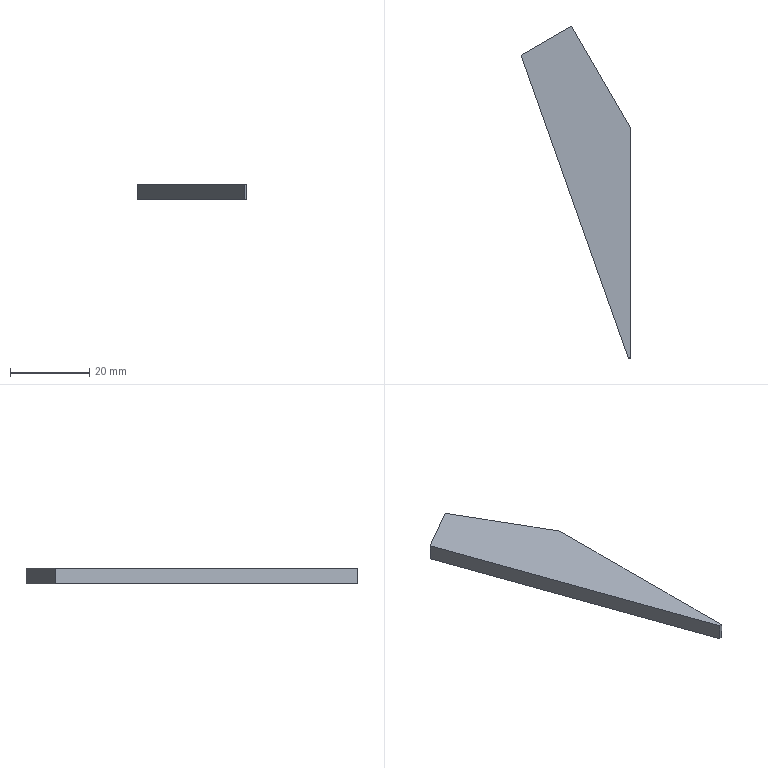Part | STEP file | Cable Chain Bracket-1 | 1 solid | 7 faces | box 27.758 x 83.881 x 4 mm | volume 4206 mm3 | plane 7
STEP:
#1=CARTESIAN_POINT('',(-31.538,-58.869,-4.));
#2=VERTEX_POINT('',#1);
#3=CARTESIAN_POINT('',(-32.245,-58.869,-4.));
#4=VERTEX_POINT('',#3);
#5=CARTESIAN_POINT('',(-32.245,-58.869,-4.));
#6=DIRECTION('',(-1.,0.,0.));
#7=VECTOR('',#6,1000.);
#8=LINE('',#5,#7);
#9=EDGE_CURVE('',#2,#4,#8,.T.);
#10=ORIENTED_EDGE('',*,*,#9,.T.);
#11=CARTESIAN_POINT('',(-59.295,17.646,-4.));
#12=VERTEX_POINT('',#11);
#13=CARTESIAN_POINT('',(-59.295,17.646,-4.));
#14=DIRECTION('',(0.3333,-0.9428,0.));
#15=VECTOR('',#14,1000.);
#16=LINE('',#13,#15);
#17=EDGE_CURVE('',#12,#4,#16,.T.);
#18=ORIENTED_EDGE('',*,*,#17,.F.);
#19=CARTESIAN_POINT('',(-46.538,25.012,-4.));
#20=VERTEX_POINT('',#19);
#21=CARTESIAN_POINT('',(-46.538,25.012,-4.));
#22=DIRECTION('',(-0.866,-0.5,0.));
#23=VECTOR('',#22,1000.);
#24=LINE('',#21,#23);
#25=EDGE_CURVE('',#20,#12,#24,.T.);
#26=ORIENTED_EDGE('',*,*,#25,.F.);
#27=CARTESIAN_POINT('',(-31.538,-0.9687,-4.));
#28=VERTEX_POINT('',#27);
#29=CARTESIAN_POINT('',(-31.538,-0.9687,-4.));
#30=DIRECTION('',(-0.5,0.866,0.));
#31=VECTOR('',#30,1000.);
#32=LINE('',#29,#31);
#33=EDGE_CURVE('',#28,#20,#32,.T.);
#34=ORIENTED_EDGE('',*,*,#33,.F.);
#35=CARTESIAN_POINT('',(-31.538,0.,-4.));
#36=DIRECTION('',(0.,1.,0.));
#37=VECTOR('',#36,1000.);
#38=LINE('',#35,#37);
#39=EDGE_CURVE('',#2,#28,#38,.T.);
#40=ORIENTED_EDGE('',*,*,#39,.F.);
#41=EDGE_LOOP('',(#10,#18,#26,#34,#40));
#42=FACE_OUTER_BOUND('',#41,.T.);
#43=CARTESIAN_POINT('',(0.,0.,-4.));
#44=DIRECTION('',(0.,0.,1.));
#45=DIRECTION('',(1.,0.,0.));
#46=AXIS2_PLACEMENT_3D('',#43,#44,#45);
#47=PLANE('',#46);
#48=ADVANCED_FACE('',(#42),#47,.F.);
#49=CARTESIAN_POINT('',(-31.538,-0.9687,0.));
#50=VERTEX_POINT('',#49);
#51=CARTESIAN_POINT('',(-31.538,-0.9687,-4.));
#52=DIRECTION('',(0.,0.,1.));
#53=VECTOR('',#52,1000.);
#54=LINE('',#51,#53);
#55=EDGE_CURVE('',#28,#50,#54,.T.);
#56=ORIENTED_EDGE('',*,*,#55,.T.);
#57=CARTESIAN_POINT('',(-31.538,-58.869,0.));
#58=VERTEX_POINT('',#57);
#59=CARTESIAN_POINT('',(-31.538,-60.869,0.));
#60=DIRECTION('',(0.,-1.,0.));
#61=VECTOR('',#60,1000.);
#62=LINE('',#59,#61);
#63=EDGE_CURVE('',#50,#58,#62,.T.);
#64=ORIENTED_EDGE('',*,*,#63,.T.);
#65=CARTESIAN_POINT('',(-31.538,-58.869,-4.));
#66=DIRECTION('',(0.,0.,-1.));
#67=VECTOR('',#66,1000.);
#68=LINE('',#65,#67);
#69=EDGE_CURVE('',#58,#2,#68,.T.);
#70=ORIENTED_EDGE('',*,*,#69,.T.);
#71=ORIENTED_EDGE('',*,*,#39,.T.);
#72=EDGE_LOOP('',(#56,#64,#70,#71));
#73=FACE_OUTER_BOUND('',#72,.T.);
#74=CARTESIAN_POINT('',(-31.538,-60.869,-4.));
#75=DIRECTION('',(1.,0.,0.));
#76=DIRECTION('',(0.,1.,0.));
#77=AXIS2_PLACEMENT_3D('',#74,#75,#76);
#78=PLANE('',#77);
#79=ADVANCED_FACE('',(#73),#78,.T.);
#80=CARTESIAN_POINT('',(-59.295,17.646,0.));
#81=VERTEX_POINT('',#80);
#82=CARTESIAN_POINT('',(-59.295,17.646,-4.));
#83=DIRECTION('',(0.,0.,-1.));
#84=VECTOR('',#83,1000.);
#85=LINE('',#82,#84);
#86=EDGE_CURVE('',#81,#12,#85,.T.);
#87=ORIENTED_EDGE('',*,*,#86,.T.);
#88=ORIENTED_EDGE('',*,*,#17,.T.);
#89=CARTESIAN_POINT('',(-32.245,-58.869,0.));
#90=VERTEX_POINT('',#89);
#91=CARTESIAN_POINT('',(-32.245,-58.869,-4.));
#92=DIRECTION('',(0.,0.,1.));
#93=VECTOR('',#92,1000.);
#94=LINE('',#91,#93);
#95=EDGE_CURVE('',#4,#90,#94,.T.);
#96=ORIENTED_EDGE('',*,*,#95,.T.);
#97=CARTESIAN_POINT('',(-59.295,17.646,0.));
#98=DIRECTION('',(-0.3333,0.9428,0.));
#99=VECTOR('',#98,1000.);
#100=LINE('',#97,#99);
#101=EDGE_CURVE('',#90,#81,#100,.T.);
#102=ORIENTED_EDGE('',*,*,#101,.T.);
#103=EDGE_LOOP('',(#87,#88,#96,#102));
#104=FACE_OUTER_BOUND('',#103,.T.);
#105=CARTESIAN_POINT('',(-59.295,17.646,-4.));
#106=DIRECTION('',(-0.9428,-0.3333,0.));
#107=DIRECTION('',(0.3333,-0.9428,0.));
#108=AXIS2_PLACEMENT_3D('',#105,#106,#107);
#109=PLANE('',#108);
#110=ADVANCED_FACE('',(#104),#109,.T.);
#111=ORIENTED_EDGE('',*,*,#25,.T.);
#112=ORIENTED_EDGE('',*,*,#86,.F.);
#113=CARTESIAN_POINT('',(-46.538,25.012,0.));
#114=VERTEX_POINT('',#113);
#115=CARTESIAN_POINT('',(-46.538,25.012,0.));
#116=DIRECTION('',(0.866,0.5,0.));
#117=VECTOR('',#116,1000.);
#118=LINE('',#115,#117);
#119=EDGE_CURVE('',#81,#114,#118,.T.);
#120=ORIENTED_EDGE('',*,*,#119,.T.);
#121=CARTESIAN_POINT('',(-46.538,25.012,-4.));
#122=DIRECTION('',(0.,0.,-1.));
#123=VECTOR('',#122,1000.);
#124=LINE('',#121,#123);
#125=EDGE_CURVE('',#114,#20,#124,.T.);
#126=ORIENTED_EDGE('',*,*,#125,.T.);
#127=EDGE_LOOP('',(#111,#112,#120,#126));
#128=FACE_OUTER_BOUND('',#127,.T.);
#129=CARTESIAN_POINT('',(-46.538,25.012,-4.));
#130=DIRECTION('',(-0.5,0.866,0.));
#131=DIRECTION('',(-0.866,-0.5,0.));
#132=AXIS2_PLACEMENT_3D('',#129,#130,#131);
#133=PLANE('',#132);
#134=ADVANCED_FACE('',(#128),#133,.T.);
#135=ORIENTED_EDGE('',*,*,#33,.T.);
#136=ORIENTED_EDGE('',*,*,#125,.F.);
#137=CARTESIAN_POINT('',(-31.538,-0.9687,0.));
#138=DIRECTION('',(0.5,-0.866,0.));
#139=VECTOR('',#138,1000.);
#140=LINE('',#137,#139);
#141=EDGE_CURVE('',#114,#50,#140,.T.);
#142=ORIENTED_EDGE('',*,*,#141,.T.);
#143=ORIENTED_EDGE('',*,*,#55,.F.);
#144=EDGE_LOOP('',(#135,#136,#142,#143));
#145=FACE_OUTER_BOUND('',#144,.T.);
#146=CARTESIAN_POINT('',(-31.538,-0.9687,-4.));
#147=DIRECTION('',(0.866,0.5,0.));
#148=DIRECTION('',(-0.5,0.866,0.));
#149=AXIS2_PLACEMENT_3D('',#146,#147,#148);
#150=PLANE('',#149);
#151=ADVANCED_FACE('',(#145),#150,.T.);
#152=ORIENTED_EDGE('',*,*,#119,.F.);
#153=ORIENTED_EDGE('',*,*,#101,.F.);
#154=CARTESIAN_POINT('',(0.,-58.869,0.));
#155=DIRECTION('',(1.,0.,0.));
#156=VECTOR('',#155,1000.);
#157=LINE('',#154,#156);
#158=EDGE_CURVE('',#90,#58,#157,.T.);
#159=ORIENTED_EDGE('',*,*,#158,.T.);
#160=ORIENTED_EDGE('',*,*,#63,.F.);
#161=ORIENTED_EDGE('',*,*,#141,.F.);
#162=EDGE_LOOP('',(#152,#153,#159,#160,#161));
#163=FACE_OUTER_BOUND('',#162,.T.);
#164=CARTESIAN_POINT('',(0.,0.,0.));
#165=DIRECTION('',(0.,0.,1.));
#166=DIRECTION('',(1.,0.,0.));
#167=AXIS2_PLACEMENT_3D('',#164,#165,#166);
#168=PLANE('',#167);
#169=ADVANCED_FACE('',(#163),#168,.T.);
#170=ORIENTED_EDGE('',*,*,#158,.F.);
#171=ORIENTED_EDGE('',*,*,#95,.F.);
#172=ORIENTED_EDGE('',*,*,#9,.F.);
#173=ORIENTED_EDGE('',*,*,#69,.F.);
#174=EDGE_LOOP('',(#170,#171,#172,#173));
#175=FACE_OUTER_BOUND('',#174,.T.);
#176=CARTESIAN_POINT('',(-32.245,-58.869,-10.));
#177=DIRECTION('',(0.,1.,0.));
#178=DIRECTION('',(-1.,0.,0.));
#179=AXIS2_PLACEMENT_3D('',#176,#177,#178);
#180=PLANE('',#179);
#181=ADVANCED_FACE('',(#175),#180,.F.);
#182=CLOSED_SHELL('',(#48,#79,#110,#134,#151,#169,#181));
#183=MANIFOLD_SOLID_BREP('',#182);
#184=CARTESIAN_POINT('',(0.,0.,0.));
#185=DIRECTION('',(0.,0.,1.));
#186=DIRECTION('',(1.,0.,0.));
#187=AXIS2_PLACEMENT_3D('',#184,#185,#186);
#188=(LENGTH_UNIT()NAMED_UNIT(*)SI_UNIT(.MILLI.,.METRE.));
#189=UNCERTAINTY_MEASURE_WITH_UNIT(LENGTH_MEASURE(0.00001),#188,'','');
#190=(NAMED_UNIT(*)PLANE_ANGLE_UNIT()SI_UNIT($,.RADIAN.));
#191=(NAMED_UNIT(*)SI_UNIT($,.STERADIAN.)SOLID_ANGLE_UNIT());
#192=(GEOMETRIC_REPRESENTATION_CONTEXT(3)GLOBAL_UNCERTAINTY_ASSIGNED_CONTEXT((#189))GLOBAL_UNIT_ASSIGNED_CONTEXT((#188,#190,#191))REPRESENTATION_CONTEXT('',''));
#193=ADVANCED_BREP_SHAPE_REPRESENTATION('',(#183,#187),#192);